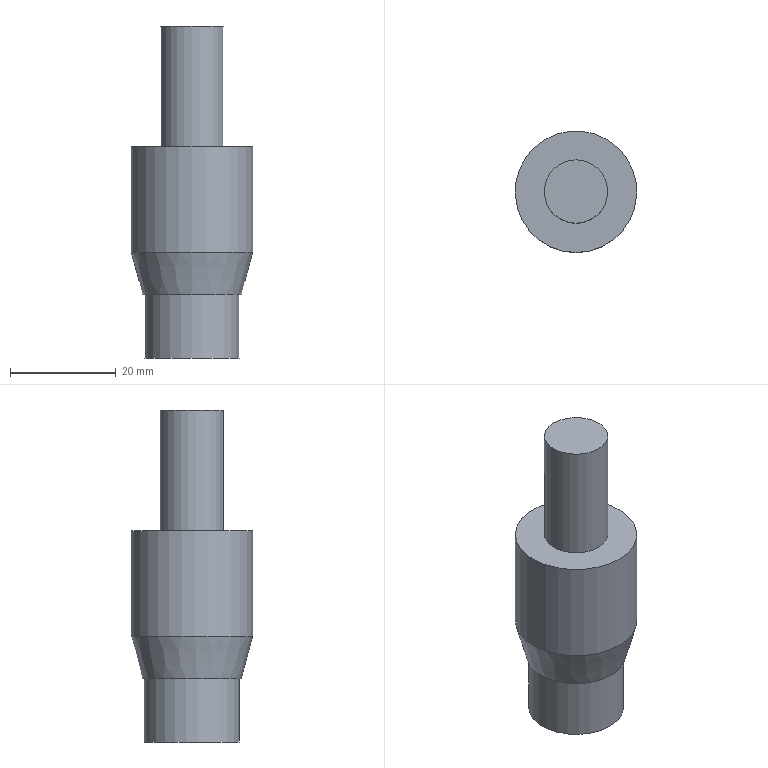Part | NX | features solid 2 | 1 solid | 8 faces | box 23 x 23 x 62.85 mm | volume 16690 mm3 | plane 4 | cylinder 3 | cone 1 | commonest cylinder face diameters 12 x1 18 x1 23 x1
STEP:
#1=CARTESIAN_POINT('',(850.,278.5,320.));
#2=VERTEX_POINT('',#1);
#3=CARTESIAN_POINT('',(850.,290.,320.));
#4=DIRECTION('',(0.,0.,-1.));
#5=DIRECTION('',(0.,-1.,0.));
#6=AXIS2_PLACEMENT_3D('',#3,#4,#5);
#7=CIRCLE('',#6,11.5);
#8=EDGE_CURVE('',#2,#2,#7,.T.);
#9=ORIENTED_EDGE('',*,*,#8,.F.);
#10=EDGE_LOOP('',(#9));
#11=FACE_BOUND('',#10,.T.);
#12=CARTESIAN_POINT('',(850.,296.,320.));
#13=VERTEX_POINT('',#12);
#14=CARTESIAN_POINT('',(850.,290.,320.));
#15=DIRECTION('',(0.,0.,1.));
#16=DIRECTION('',(0.,1.,0.));
#17=AXIS2_PLACEMENT_3D('',#14,#15,#16);
#18=CIRCLE('',#17,6.);
#19=EDGE_CURVE('',#13,#13,#18,.T.);
#20=ORIENTED_EDGE('',*,*,#19,.F.);
#21=EDGE_LOOP('',(#20));
#22=FACE_BOUND('',#21,.T.);
#23=CARTESIAN_POINT('',(850.,290.,320.));
#24=DIRECTION('',(0.,0.,1.));
#25=DIRECTION('',(0.,1.,0.));
#26=AXIS2_PLACEMENT_3D('',#23,#24,#25);
#27=PLANE('',#26);
#28=ADVANCED_FACE('',(#11,#22),#27,.T.);
#29=CARTESIAN_POINT('',(850.,280.644,292.));
#30=VERTEX_POINT('',#29);
#31=CARTESIAN_POINT('',(850.,290.,292.));
#32=DIRECTION('',(0.,0.,-1.));
#33=DIRECTION('',(0.,-1.,0.));
#34=AXIS2_PLACEMENT_3D('',#31,#32,#33);
#35=CIRCLE('',#34,9.356);
#36=EDGE_CURVE('',#30,#30,#35,.T.);
#37=ORIENTED_EDGE('',*,*,#36,.T.);
#38=EDGE_LOOP('',(#37));
#39=FACE_BOUND('',#38,.T.);
#40=CARTESIAN_POINT('',(850.,281.,292.));
#41=VERTEX_POINT('',#40);
#42=CARTESIAN_POINT('',(850.,290.,292.));
#43=DIRECTION('',(0.,0.,-1.));
#44=DIRECTION('',(0.,-1.,0.));
#45=AXIS2_PLACEMENT_3D('',#42,#43,#44);
#46=CIRCLE('',#45,9.);
#47=EDGE_CURVE('',#41,#41,#46,.T.);
#48=ORIENTED_EDGE('',*,*,#47,.F.);
#49=EDGE_LOOP('',(#48));
#50=FACE_BOUND('',#49,.T.);
#51=CARTESIAN_POINT('',(850.,290.,292.));
#52=DIRECTION('',(0.,0.,-1.));
#53=DIRECTION('',(0.,-1.,0.));
#54=AXIS2_PLACEMENT_3D('',#51,#52,#53);
#55=PLANE('',#54);
#56=ADVANCED_FACE('',(#39,#50),#55,.T.);
#57=CARTESIAN_POINT('',(850.,278.5,300.));
#58=VERTEX_POINT('',#57);
#59=CARTESIAN_POINT('',(850.,290.,300.));
#60=DIRECTION('',(0.,0.,-1.));
#61=DIRECTION('',(0.,-1.,0.));
#62=AXIS2_PLACEMENT_3D('',#59,#60,#61);
#63=CIRCLE('',#62,11.5);
#64=EDGE_CURVE('',#58,#58,#63,.F.);
#65=ORIENTED_EDGE('',*,*,#64,.T.);
#66=EDGE_LOOP('',(#65));
#67=FACE_BOUND('',#66,.T.);
#68=ORIENTED_EDGE('',*,*,#8,.T.);
#69=EDGE_LOOP('',(#68));
#70=FACE_BOUND('',#69,.T.);
#71=CARTESIAN_POINT('',(850.,290.,320.));
#72=DIRECTION('',(0.,0.,-1.));
#73=DIRECTION('',(0.,-1.,0.));
#74=AXIS2_PLACEMENT_3D('',#71,#72,#73);
#75=CYLINDRICAL_SURFACE('',#74,11.5);
#76=ADVANCED_FACE('',(#67,#70),#75,.T.);
#77=ORIENTED_EDGE('',*,*,#19,.T.);
#78=EDGE_LOOP('',(#77));
#79=FACE_BOUND('',#78,.T.);
#80=CARTESIAN_POINT('',(850.,284.,342.85));
#81=VERTEX_POINT('',#80);
#82=CARTESIAN_POINT('',(850.,290.,342.85));
#83=DIRECTION('',(0.,0.,-1.));
#84=DIRECTION('',(0.,-1.,0.));
#85=AXIS2_PLACEMENT_3D('',#82,#83,#84);
#86=CIRCLE('',#85,6.);
#87=EDGE_CURVE('',#81,#81,#86,.F.);
#88=ORIENTED_EDGE('',*,*,#87,.F.);
#89=EDGE_LOOP('',(#88));
#90=FACE_BOUND('',#89,.T.);
#91=CARTESIAN_POINT('',(850.,290.,308.75));
#92=DIRECTION('',(0.,0.,-1.));
#93=DIRECTION('',(0.,-1.,0.));
#94=AXIS2_PLACEMENT_3D('',#91,#92,#93);
#95=CYLINDRICAL_SURFACE('',#94,6.);
#96=ADVANCED_FACE('',(#79,#90),#95,.T.);
#97=ORIENTED_EDGE('',*,*,#87,.T.);
#98=EDGE_LOOP('',(#97));
#99=FACE_BOUND('',#98,.T.);
#100=CARTESIAN_POINT('',(850.,290.,342.85));
#101=DIRECTION('',(0.,0.,-1.));
#102=DIRECTION('',(0.,-1.,0.));
#103=AXIS2_PLACEMENT_3D('',#100,#101,#102);
#104=PLANE('',#103);
#105=ADVANCED_FACE('',(#99),#104,.F.);
#106=CARTESIAN_POINT('',(850.,299.,280.));
#107=VERTEX_POINT('',#106);
#108=CARTESIAN_POINT('',(850.,290.,280.));
#109=DIRECTION('',(0.,0.,1.));
#110=DIRECTION('',(0.,1.,0.));
#111=AXIS2_PLACEMENT_3D('',#108,#109,#110);
#112=CIRCLE('',#111,9.);
#113=EDGE_CURVE('',#107,#107,#112,.T.);
#114=ORIENTED_EDGE('',*,*,#113,.F.);
#115=EDGE_LOOP('',(#114));
#116=FACE_BOUND('',#115,.T.);
#117=CARTESIAN_POINT('',(850.,290.,280.));
#118=DIRECTION('',(0.,0.,-1.));
#119=DIRECTION('',(0.,-1.,0.));
#120=AXIS2_PLACEMENT_3D('',#117,#118,#119);
#121=PLANE('',#120);
#122=ADVANCED_FACE('',(#116),#121,.T.);
#123=ORIENTED_EDGE('',*,*,#113,.T.);
#124=EDGE_LOOP('',(#123));
#125=FACE_BOUND('',#124,.T.);
#126=ORIENTED_EDGE('',*,*,#47,.T.);
#127=EDGE_LOOP('',(#126));
#128=FACE_BOUND('',#127,.T.);
#129=CARTESIAN_POINT('',(850.,290.,292.));
#130=DIRECTION('',(0.,0.,-1.));
#131=DIRECTION('',(0.,-1.,0.));
#132=AXIS2_PLACEMENT_3D('',#129,#130,#131);
#133=CYLINDRICAL_SURFACE('',#132,9.);
#134=ADVANCED_FACE('',(#125,#128),#133,.T.);
#135=ORIENTED_EDGE('',*,*,#36,.F.);
#136=EDGE_LOOP('',(#135));
#137=FACE_BOUND('',#136,.T.);
#138=ORIENTED_EDGE('',*,*,#64,.F.);
#139=EDGE_LOOP('',(#138));
#140=FACE_BOUND('',#139,.T.);
#141=CARTESIAN_POINT('',(850.,290.,300.));
#142=DIRECTION('',(0.,0.,1.));
#143=DIRECTION('',(0.,1.,0.));
#144=AXIS2_PLACEMENT_3D('',#141,#142,#143);
#145=CONICAL_SURFACE('',#144,11.5,0.2618);
#146=ADVANCED_FACE('',(#137,#140),#145,.T.);
#147=CLOSED_SHELL('',(#28,#56,#76,#96,#105,#122,#134,#146));
#148=MANIFOLD_SOLID_BREP('',#147);
#149=(LENGTH_UNIT()NAMED_UNIT(*)SI_UNIT(.MILLI.,.METRE.));
#150=UNCERTAINTY_MEASURE_WITH_UNIT(LENGTH_MEASURE(0.00001),#149,'','');
#151=(NAMED_UNIT(*)PLANE_ANGLE_UNIT()SI_UNIT($,.RADIAN.));
#152=(NAMED_UNIT(*)SI_UNIT($,.STERADIAN.)SOLID_ANGLE_UNIT());
#153=(GEOMETRIC_REPRESENTATION_CONTEXT(3)GLOBAL_UNCERTAINTY_ASSIGNED_CONTEXT((#150))GLOBAL_UNIT_ASSIGNED_CONTEXT((#149,#151,#152))REPRESENTATION_CONTEXT('',''));
#154=ADVANCED_BREP_SHAPE_REPRESENTATION('',(#148),#153);